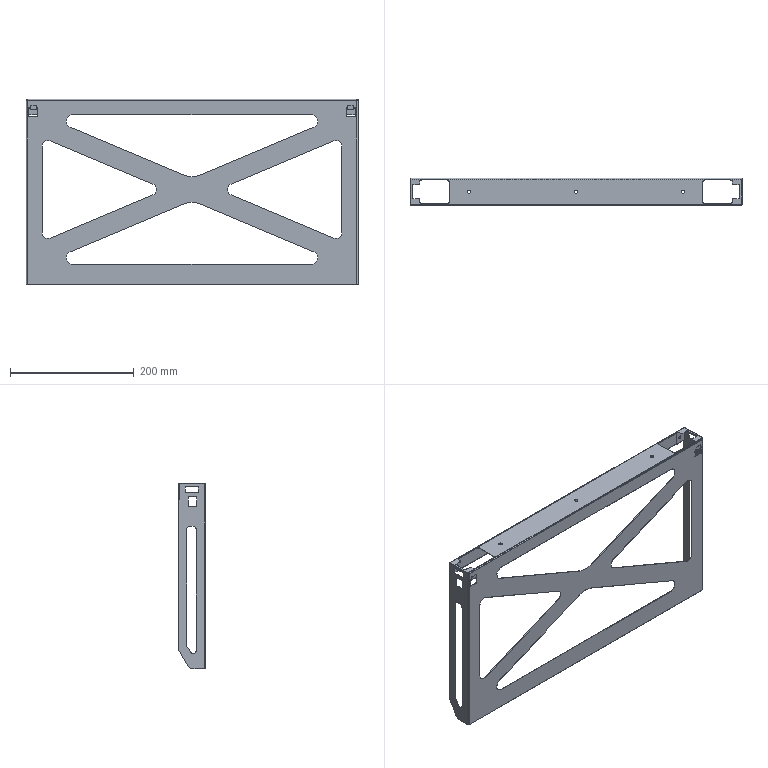Part | NX | features solid 2 | 1 solid | 248 faces | box 537 x 45.1 x 300 mm | volume 103075 mm3 | cylinder 116 | plane 112 | torus 16 | cone 4 | commonest cylinder face diameters 2 x28 0.2 x18 1 x16 5 x12 10.102 x8 5.2 x6